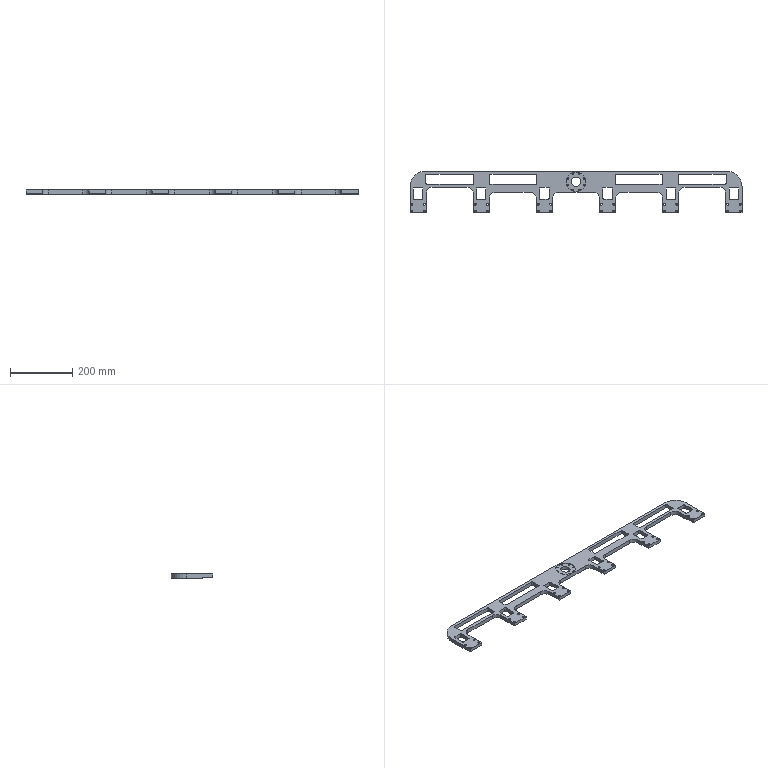NC program | NX | posted with a generic post | part box 1068 x 134 x 13 mm
Lines 1285 to 2457 of 4175:
(ZLEVEL_PROFILE_COPY_1_COPY_COPY , TOOL : D6)
N2526 T06 M6
N2528 G54
N2530 G17 G0 G90 X477.721 Y29.2 S9500 M3
N2532 G43 Z30. H6
N2534 Z-0.591
N2536 G94 G1 Y28.003 F1000.
N2538 X477.784 Y28.
N2540 X480. F1650.
N2542 Y30.216
N2544 X479.997 Y30.279
N2546 X478.8
N2548 G0 X477.721 Y29.2 Z-1.182
N2550 G1 Y28.003 F1000.
N2552 X477.784 Y28.
N2554 X480. F1650.
N2556 Y30.216
N2558 X479.997 Y30.279
N2560 X478.8
N2562 G0 X477.721 Y29.2 Z-1.773
N2564 G1 Y28.003 F1000.
N2566 X477.784 Y28.
N2568 X480. F1650.
N2570 Y30.216
N2572 X479.997 Y30.279
N2574 X478.8
N2576 G0 X477.721 Y29.2 Z-2.364
N2578 G1 Y28.003 F1000.
N2580 X477.784 Y28.
N2582 X480. F1650.
N2584 Y30.216
N2586 X479.997 Y30.279
N2588 X478.8
N2590 G0 X477.721 Y29.2 Z-2.955
N2592 G1 Y28.003 F1000.
N2594 X477.784 Y28.
N2596 X480. F1650.
N2598 Y30.216
N2600 X479.997 Y30.279
N2602 X478.8
N2604 G0 X477.721 Y29.2 Z-3.545
N2606 G1 Y28.003 F1000.
N2608 X477.784 Y28.
N2610 X480. F1650.
N2612 Y30.216
N2614 X479.997 Y30.279
N2616 X478.8
N2618 G0 X477.721 Y29.2 Z-4.136
N2620 G1 Y28.003 F1000.
N2622 X477.784 Y28.
N2624 X480. F1650.
N2626 Y30.216
N2628 X479.997 Y30.279
N2630 X478.8
N2632 G0 X477.721 Y29.2 Z-4.727
N2634 G1 Y28.003 F1000.
N2636 X477.784 Y28.
N2638 X480. F1650.
N2640 Y30.216
N2642 X479.997 Y30.279
N2644 X478.8
N2646 G0 X477.721 Y29.2 Z-5.318
N2648 G1 Y28.003 F1000.
N2650 X477.784 Y28.
N2652 X480. F1650.
N2654 Y30.216
N2656 X479.997 Y30.279
N2658 X478.8
N2660 G0 X477.721 Y29.2 Z-5.909
N2662 G1 Y28.003 F1000.
N2664 X477.784 Y28.
N2666 X480. F1650.
N2668 Y30.216
N2670 X479.997 Y30.279
N2672 X478.8
N2674 G0 X477.721 Y29.2 Z-6.5
N2676 G1 Y28.003 F1000.
N2678 X477.784 Y28.
N2680 X480. F1650.
N2682 Y30.216
N2684 X479.997 Y30.279
N2686 X478.8
N2688 G0 X477.721 Y29.2 Z-7.091
N2690 G1 Y28.003 F1000.
N2692 X477.784 Y28.
N2694 X480. F1650.
N2696 Y30.216
N2698 X479.997 Y30.279
N2700 X478.8
N2702 G0 X477.721 Y29.2 Z-7.682
N2704 G1 Y28.003 F1000.
N2706 X477.784 Y28.
N2708 X480. F1650.
N2710 Y30.216
N2712 X479.997 Y30.279
N2714 X478.8
N2716 G0 X477.709 Y29.2 Z-8.273
N2718 G1 Y28.003 F1000.
N2720 X477.772 Y28.
N2722 X480. F1650.
N2724 Y30.218
N2726 X479.997 Y30.281
N2728 X478.8
N2730 G0 X477.709 Y29.2 Z-8.864
N2732 G1 Y28.003 F1000.
N2734 X477.772 Y28.
N2736 X480. F1650.
N2738 Y30.218
N2740 X479.997 Y30.281
N2742 X478.8
N2744 G0 X477.709 Y29.2 Z-9.455
N2746 G1 Y28.003 F1000.
N2748 X477.772 Y28.
N2750 X480. F1650.
N2752 Y30.218
N2754 X479.997 Y30.281
N2756 X478.8
N2758 G0 X477.709 Y29.2 Z-10.045
N2760 G1 Y28.003 F1000.
N2762 X477.772 Y28.
N2764 X480. F1650.
N2766 Y30.218
N2768 X479.997 Y30.281
N2770 X478.8
N2772 G0 X477.709 Y29.2 Z-10.636
N2774 G1 Y28.003 F1000.
N2776 X477.772 Y28.
N2778 X480. F1650.
N2780 Y30.218
N2782 X479.997 Y30.281
N2784 X478.8
N2786 G0 X477.709 Y29.2 Z-11.227
N2788 G1 Y28.003 F1000.
N2790 X477.772 Y28.
N2792 X480. F1650.
N2794 Y30.218
N2796 X479.997 Y30.281
N2798 X478.8
N2800 G0 X477.709 Y29.2 Z-11.818
N2802 G1 Y28.003 F1000.
N2804 X477.772 Y28.
N2806 X480. F1650.
N2808 Y30.218
N2810 X479.997 Y30.281
N2812 X478.8
N2814 G0 X477.709 Y29.2 Z-12.409
N2816 G1 Y28.003 F1000.
N2818 X477.772 Y28.
N2820 X480. F1650.
N2822 Y30.218
N2824 X479.997 Y30.281
N2826 X478.8
N2828 G0 X477.709 Y29.2 Z-13.
N2830 G1 Y28.003 F1000.
N2832 X477.772 Y28.
N2834 X480. F1650.
N2836 Y30.218
N2838 X479.997 Y30.281
N2840 X478.8
N2842 G0 Z30.
N2844 Y51.721
N2846 Z-0.591
N2848 G1 X479.997 F1000.
N2850 X480. Y51.784
N2852 Y54. F1650.
N2854 X477.784
N2856 X477.721 Y53.997
N2858 Y52.8
N2860 G0 X478.8 Y51.721 Z-1.182
N2862 G1 X479.997 F1000.
N2864 X480. Y51.784
N2866 Y54. F1650.
N2868 X477.784
N2870 X477.721 Y53.997
N2872 Y52.8
N2874 G0 X478.8 Y51.721 Z-1.773
N2876 G1 X479.997 F1000.
N2878 X480. Y51.784
N2880 Y54. F1650.
N2882 X477.784
N2884 X477.721 Y53.997
N2886 Y52.8
N2888 G0 X478.8 Y51.721 Z-2.364
N2890 G1 X479.997 F1000.
N2892 X480. Y51.784
N2894 Y54. F1650.
N2896 X477.784
N2898 X477.721 Y53.997
N2900 Y52.8
N2902 G0 X478.8 Y51.721 Z-2.955
N2904 G1 X479.997 F1000.
N2906 X480. Y51.784
N2908 Y54. F1650.
N2910 X477.784
N2912 X477.721 Y53.997
N2914 Y52.8
N2916 G0 X478.8 Y51.721 Z-3.545
N2918 G1 X479.997 F1000.
N2920 X480. Y51.784
N2922 Y54. F1650.
N2924 X477.784
N2926 X477.721 Y53.997
N2928 Y52.8
N2930 G0 X478.8 Y51.721 Z-4.136
N2932 G1 X479.997 F1000.
N2934 X480. Y51.784
N2936 Y54. F1650.
N2938 X477.784
N2940 X477.721 Y53.997
N2942 Y52.8
N2944 G0 X478.8 Y51.721 Z-4.727
N2946 G1 X479.997 F1000.
N2948 X480. Y51.784
N2950 Y54. F1650.
N2952 X477.784
N2954 X477.721 Y53.997
N2956 Y52.8
N2958 G0 X478.8 Y51.721 Z-5.318
N2960 G1 X479.997 F1000.
N2962 X480. Y51.784
N2964 Y54. F1650.
N2966 X477.784
N2968 X477.721 Y53.997
N2970 Y52.8
N2972 G0 X478.8 Y51.721 Z-5.909
N2974 G1 X479.997 F1000.
N2976 X480. Y51.784
N2978 Y54. F1650.
N2980 X477.784
N2982 X477.721 Y53.997
N2984 Y52.8
N2986 G0 X478.8 Y51.721 Z-6.5
N2988 G1 X479.997 F1000.
N2990 X480. Y51.784
N2992 Y54. F1650.
N2994 X477.784
N2996 X477.721 Y53.997
N2998 Y52.8
N3000 G0 X478.8 Y51.721 Z-7.091
N3002 G1 X479.997 F1000.
N3004 X480. Y51.784
N3006 Y54. F1650.
N3008 X477.784
N3010 X477.721 Y53.997
N3012 Y52.8
N3014 G0 X478.8 Y51.721 Z-7.682
N3016 G1 X479.997 F1000.
N3018 X480. Y51.784
N3020 Y54. F1650.
N3022 X477.784
N3024 X477.721 Y53.997
N3026 Y52.8
N3028 G0 X478.8 Y51.73 Z-8.273
N3030 G1 X479.997 F1000.
N3032 X480. Y51.793
N3034 Y53.988 F1650.
N3036 Y54.
N3038 X477.795
N3040 X477.732 Y53.997
N3042 Y52.8
N3044 G0 X478.8 Y51.73 Z-8.864
N3046 G1 X479.997 F1000.
N3048 X480. Y51.793
N3050 Y53.988 F1650.
N3052 Y54.
N3054 X477.795
N3056 X477.732 Y53.997
N3058 Y52.8
N3060 G0 X478.8 Y51.73 Z-9.455
N3062 G1 X479.997 F1000.
N3064 X480. Y51.793
N3066 Y53.988 F1650.
N3068 Y54.
N3070 X477.795
N3072 X477.732 Y53.997
N3074 Y52.8
N3076 G0 X478.8 Y51.73 Z-10.045
N3078 G1 X479.997 F1000.
N3080 X480. Y51.793
N3082 Y53.988 F1650.
N3084 Y54.
N3086 X477.795
N3088 X477.732 Y53.997
N3090 Y52.8
N3092 G0 X478.8 Y51.73 Z-10.636
N3094 G1 X479.997 F1000.
N3096 X480. Y51.793
N3098 Y53.988 F1650.
N3100 Y54.
N3102 X477.795
N3104 X477.732 Y53.997
N3106 Y52.8
N3108 G0 X478.8 Y51.73 Z-11.227
N3110 G1 X479.997 F1000.
N3112 X480. Y51.793
N3114 Y53.988 F1650.
N3116 Y54.
N3118 X477.795
N3120 X477.732 Y53.997
N3122 Y52.8
N3124 G0 X478.8 Y51.73 Z-11.818
N3126 G1 X479.997 F1000.
N3128 X480. Y51.793
N3130 Y53.988 F1650.
N3132 Y54.
N3134 X477.795
N3136 X477.732 Y53.997
N3138 Y52.8
N3140 G0 X478.8 Y51.73 Z-12.409
N3142 G1 X479.997 F1000.
N3144 X480. Y51.793
N3146 Y53.988 F1650.
N3148 Y54.
N3150 X477.795
N3152 X477.732 Y53.997
N3154 Y52.8
N3156 G0 X478.8 Y51.73 Z-13.
N3158 G1 X479.997 F1000.
N3160 X480. Y51.793
N3162 Y53.988 F1650.
N3164 Y54.
N3166 X477.795
N3168 X477.732 Y53.997
N3170 Y52.8
N3172 G0 Z30.
N3174 X335.079
N3176 Z-0.591
N3178 G1 Y53.997 F1000.
N3180 X335.016 Y54.
N3182 X332.8 F1650.
N3184 Y51.784
N3186 X332.803 Y51.721
N3188 X334.
N3190 G0 X335.079 Y52.8 Z-1.182
N3192 G1 Y53.997 F1000.
N3194 X335.016 Y54.
N3196 X332.8 F1650.
N3198 Y51.784
N3200 X332.803 Y51.721
N3202 X334.
N3204 G0 X335.079 Y52.8 Z-1.773
N3206 G1 Y53.997 F1000.
N3208 X335.016 Y54.
N3210 X332.8 F1650.
N3212 Y51.784
N3214 X332.803 Y51.721
N3216 X334.
N3218 G0 X335.079 Y52.8 Z-2.364
N3220 G1 Y53.997 F1000.
N3222 X335.016 Y54.
N3224 X332.8 F1650.
N3226 Y51.784
N3228 X332.803 Y51.721
N3230 X334.
N3232 G0 X335.079 Y52.8 Z-2.955
N3234 G1 Y53.997 F1000.
N3236 X335.016 Y54.
N3238 X332.8 F1650.
N3240 Y51.784
N3242 X332.803 Y51.721
N3244 X334.
N3246 G0 X335.079 Y52.8 Z-3.545
N3248 G1 Y53.997 F1000.
N3250 X335.016 Y54.
N3252 X332.8 F1650.
N3254 Y51.784
N3256 X332.803 Y51.721
N3258 X334.
N3260 G0 X335.079 Y52.8 Z-4.136
N3262 G1 Y53.997 F1000.
N3264 X335.016 Y54.
N3266 X332.8 F1650.
N3268 Y51.784
N3270 X332.803 Y51.721
N3272 X334.
N3274 G0 X335.079 Y52.8 Z-4.727
N3276 G1 Y53.997 F1000.
N3278 X335.016 Y54.
N3280 X332.8 F1650.
N3282 Y51.784
N3284 X332.803 Y51.721
N3286 X334.
N3288 G0 X335.079 Y52.8 Z-5.318
N3290 G1 Y53.997 F1000.
N3292 X335.016 Y54.
N3294 X332.8 F1650.
N3296 Y51.784
N3298 X332.803 Y51.721
N3300 X334.
N3302 G0 X335.079 Y52.8 Z-5.909
N3304 G1 Y53.997 F1000.
N3306 X335.016 Y54.
N3308 X332.8 F1650.
N3310 Y51.784
N3312 X332.803 Y51.721
N3314 X334.
N3316 G0 X335.079 Y52.8 Z-6.5
N3318 G1 Y53.997 F1000.
N3320 X335.016 Y54.
N3322 X332.8 F1650.
N3324 Y51.784
N3326 X332.803 Y51.721
N3328 X334.
N3330 G0 X335.079 Y52.8 Z-7.091
N3332 G1 Y53.997 F1000.
N3334 X335.016 Y54.
N3336 X332.8 F1650.
N3338 Y51.784
N3340 X332.803 Y51.721
N3342 X334.
N3344 G0 X335.079 Y52.8 Z-7.682
N3346 G1 Y53.997 F1000.
N3348 X335.016 Y54.
N3350 X332.8 F1650.
N3352 Y51.784
N3354 X332.803 Y51.721
N3356 X334.
N3358 G0 X335.076 Y52.8 Z-8.273
N3360 G1 Y53.997 F1000.
N3362 X335.013 Y54.
N3364 X332.8 F1650.
N3366 Y51.774
N3368 X332.803 Y51.711
N3370 X334.
N3372 G0 X335.076 Y52.8 Z-8.864
N3374 G1 Y53.997 F1000.
N3376 X335.013 Y54.
N3378 X332.8 F1650.
N3380 Y51.774
N3382 X332.803 Y51.711
N3384 X334.
N3386 G0 X335.076 Y52.8 Z-9.455
N3388 G1 Y53.997 F1000.
N3390 X335.013 Y54.
N3392 X332.8 F1650.
N3394 Y51.774
N3396 X332.803 Y51.711
N3398 X334.
N3400 G0 X335.076 Y52.8 Z-10.045
N3402 G1 Y53.997 F1000.
N3404 X335.013 Y54.
N3406 X332.8 F1650.
N3408 Y51.774
N3410 X332.803 Y51.711
N3412 X334.
N3414 G0 X335.076 Y52.8 Z-10.636
N3416 G1 Y53.997 F1000.
N3418 X335.013 Y54.
N3420 X332.8 F1650.
N3422 Y51.774
N3424 X332.803 Y51.711
N3426 X334.
N3428 G0 X335.076 Y52.8 Z-11.227
N3430 G1 Y53.997 F1000.
N3432 X335.013 Y54.
N3434 X332.8 F1650.
N3436 Y51.774
N3438 X332.803 Y51.711
N3440 X334.
N3442 G0 X335.076 Y52.8 Z-11.818
N3444 G1 Y53.997 F1000.
N3446 X335.013 Y54.
N3448 X332.8 F1650.
N3450 Y51.774
N3452 X332.803 Y51.711
N3454 X334.
N3456 G0 X335.076 Y52.8 Z-12.409
N3458 G1 Y53.997 F1000.
N3460 X335.013 Y54.
N3462 X332.8 F1650.
N3464 Y51.774
N3466 X332.803 Y51.711
N3468 X334.
N3470 G0 X335.076 Y52.8 Z-13.
N3472 G1 Y53.997 F1000.
N3474 X335.013 Y54.
N3476 X332.8 F1650.
N3478 Y51.774
N3480 X332.803 Y51.711
N3482 X334.
N3484 G0 Z30.
N3486 Y30.279
N3488 Z-0.591
N3490 G1 X332.803 F1000.
N3492 X332.8 Y30.216
N3494 Y28. F1650.
N3496 X335.016
N3498 X335.079 Y28.003
N3500 Y29.2
N3502 G0 X334. Y30.279 Z-1.182
N3504 G1 X332.803 F1000.
N3506 X332.8 Y30.216
N3508 Y28. F1650.
N3510 X335.016
N3512 X335.079 Y28.003
N3514 Y29.2
N3516 G0 X334. Y30.279 Z-1.773
N3518 G1 X332.803 F1000.
N3520 X332.8 Y30.216
N3522 Y28. F1650.
N3524 X335.016
N3526 X335.079 Y28.003
N3528 Y29.2
N3530 G0 X334. Y30.279 Z-2.364
N3532 G1 X332.803 F1000.
N3534 X332.8 Y30.216
N3536 Y28. F1650.
N3538 X335.016
N3540 X335.079 Y28.003
N3542 Y29.2
N3544 G0 X334. Y30.279 Z-2.955
N3546 G1 X332.803 F1000.
N3548 X332.8 Y30.216
N3550 Y28. F1650.
N3552 X335.016
N3554 X335.079 Y28.003
N3556 Y29.2
N3558 G0 X334. Y30.279 Z-3.545
N3560 G1 X332.803 F1000.
N3562 X332.8 Y30.216
N3564 Y28. F1650.
N3566 X335.016
N3568 X335.079 Y28.003
N3570 Y29.2
N3572 G0 X334. Y30.279 Z-4.136
N3574 G1 X332.803 F1000.
N3576 X332.8 Y30.216
N3578 Y28. F1650.
N3580 X335.016
N3582 X335.079 Y28.003
N3584 Y29.2
N3586 G0 X334. Y30.279 Z-4.727
N3588 G1 X332.803 F1000.
N3590 X332.8 Y30.216
N3592 Y28. F1650.
N3594 X335.016
N3596 X335.079 Y28.003
N3598 Y29.2
N3600 G0 X334. Y30.279 Z-5.318
N3602 G1 X332.803 F1000.
N3604 X332.8 Y30.216
N3606 Y28. F1650.
N3608 X335.016
N3610 X335.079 Y28.003
N3612 Y29.2
N3614 G0 X334. Y30.279 Z-5.909
N3616 G1 X332.803 F1000.
N3618 X332.8 Y30.216
N3620 Y28. F1650.
N3622 X335.016
N3624 X335.079 Y28.003
N3626 Y29.2
N3628 G0 X334. Y30.279 Z-6.5
N3630 G1 X332.803 F1000.
N3632 X332.8 Y30.216
N3634 Y28. F1650.
N3636 X335.016
N3638 X335.079 Y28.003
N3640 Y29.2
N3642 G0 X334. Y30.279 Z-7.091
N3644 G1 X332.803 F1000.
N3646 X332.8 Y30.216
N3648 Y28. F1650.
N3650 X335.016
N3652 X335.079 Y28.003
N3654 Y29.2
N3656 G0 X334. Y30.279 Z-7.682
N3658 G1 X332.803 F1000.
N3660 X332.8 Y30.216
N3662 Y28. F1650.
N3664 X335.016
N3666 X335.079 Y28.003
N3668 Y29.2
N3670 G0 X334. Y30.279 Z-8.273
N3672 G1 X332.803 F1000.
N3674 X332.8 Y30.216
N3676 Y28. F1650.
N3678 X335.016
N3680 X335.079 Y28.003
N3682 Y29.2
N3684 G0 X334. Y30.279 Z-8.864
N3686 G1 X332.803 F1000.
N3688 X332.8 Y30.216
N3690 Y28. F1650.
N3692 X335.016
N3694 X335.079 Y28.003
N3696 Y29.2
N3698 G0 X334. Y30.279 Z-9.455
N3700 G1 X332.803 F1000.
N3702 X332.8 Y30.216
N3704 Y28. F1650.
N3706 X335.016
N3708 X335.079 Y28.003
N3710 Y29.2
N3712 G0 X334. Y30.279 Z-10.045
N3714 G1 X332.803 F1000.
N3716 X332.8 Y30.216
N3718 Y28. F1650.
N3720 X335.016
N3722 X335.079 Y28.003
N3724 Y29.2
N3726 G0 X334. Y30.279 Z-10.636
N3728 G1 X332.803 F1000.
N3730 X332.8 Y30.216
N3732 Y28. F1650.
N3734 X335.016
N3736 X335.079 Y28.003
N3738 Y29.2
N3740 G0 X334. Y30.279 Z-11.227
N3742 G1 X332.803 F1000.
N3744 X332.8 Y30.216
N3746 Y28. F1650.
N3748 X335.016
N3750 X335.079 Y28.003
N3752 Y29.2
N3754 G0 X334. Y30.279 Z-11.818
N3756 G1 X332.803 F1000.
N3758 X332.8 Y30.216
N3760 Y28. F1650.
N3762 X335.016
N3764 X335.079 Y28.003
N3766 Y29.2
N3768 G0 X334. Y30.279 Z-12.409
N3770 G1 X332.803 F1000.
N3772 X332.8 Y30.216
N3774 Y28. F1650.
N3776 X335.016
N3778 X335.079 Y28.003
N3780 Y29.2
N3782 G0 X334. Y30.279 Z-13.
N3784 G1 X332.803 F1000.
N3786 X332.8 Y30.216
N3788 Y28. F1650.
N3790 X335.016
N3792 X335.079 Y28.003
N3794 Y29.2
N3796 G0 Z30.
N3798 X274.521
N3800 Z-0.591
N3802 G1 Y28.003 F1000.
N3804 X274.584 Y28.
N3806 X276.8 F1650.
N3808 Y30.216
N3810 X276.797 Y30.279
N3812 X275.6
N3814 G0 X274.521 Y29.2 Z-1.182
N3816 G1 Y28.003 F1000.
N3818 X274.584 Y28.
N3820 X276.8 F1650.
N3822 Y30.216
N3824 X276.797 Y30.279
N3826 X275.6
N3828 G0 X274.521 Y29.2 Z-1.773
N3830 G1 Y28.003 F1000.
N3832 X274.584 Y28.
N3834 X276.8 F1650.
N3836 Y30.216
N3838 X276.797 Y30.279
N3840 X275.6
N3842 G0 X274.521 Y29.2 Z-2.364
N3844 G1 Y28.003 F1000.
N3846 X274.584 Y28.
N3848 X276.8 F1650.
N3850 Y30.216
N3852 X276.797 Y30.279
N3854 X275.6
N3856 G0 X274.521 Y29.2 Z-2.955
N3858 G1 Y28.003 F1000.
N3860 X274.584 Y28.
N3862 X276.8 F1650.
N3864 Y30.216
N3866 X276.797 Y30.279
N3868 X275.6
N3870 G0 X274.521 Y29.2 Z-3.545
N3872 G1 Y28.003 F1000.
N3874 X274.584 Y28.
N3876 X276.8 F1650.
N3878 Y30.216
N3880 X276.797 Y30.279
N3882 X275.6
N3884 G0 X274.521 Y29.2 Z-4.136
N3886 G1 Y28.003 F1000.
N3888 X274.584 Y28.
N3890 X276.8 F1650.
N3892 Y30.216
N3894 X276.797 Y30.279
N3896 X275.6
N3898 G0 X274.521 Y29.2 Z-4.727
N3900 G1 Y28.003 F1000.
N3902 X274.584 Y28.
N3904 X276.8 F1650.
N3906 Y30.216
N3908 X276.797 Y30.279
N3910 X275.6
N3912 G0 X274.521 Y29.2 Z-5.318
N3914 G1 Y28.003 F1000.
N3916 X274.584 Y28.
N3918 X276.8 F1650.
N3920 Y30.216
N3922 X276.797 Y30.279
N3924 X275.6
N3926 G0 X274.521 Y29.2 Z-5.909
N3928 G1 Y28.003 F1000.
N3930 X274.584 Y28.
N3932 X276.8 F1650.
N3934 Y30.216
N3936 X276.797 Y30.279
N3938 X275.6
N3940 G0 X274.521 Y29.2 Z-6.5
N3942 G1 Y28.003 F1000.
N3944 X274.584 Y28.
N3946 X276.8 F1650.
N3948 Y30.216
N3950 X276.797 Y30.279
N3952 X275.6
N3954 G0 X274.521 Y29.2 Z-7.091
N3956 G1 Y28.003 F1000.
N3958 X274.584 Y28.
N3960 X276.8 F1650.
N3962 Y30.216
N3964 X276.797 Y30.279
N3966 X275.6
N3968 G0 X274.521 Y29.2 Z-7.682
N3970 G1 Y28.003 F1000.
N3972 X274.584 Y28.
N3974 X276.8 F1650.
N3976 Y30.216
N3978 X276.797 Y30.279
N3980 X275.6
N3982 G0 X274.507 Y29.2 Z-8.273
N3984 G1 Y28.003 F1000.
N3986 X274.569 Y28.
N3988 X276.8 F1650.
N3990 Y30.217
N3992 X276.797 Y30.28
N3994 X275.6
N3996 G0 X274.507 Y29.2 Z-8.864
N3998 G1 Y28.003 F1000.
N4000 X274.569 Y28.
N4002 X276.8 F1650.
N4004 Y30.217
N4006 X276.797 Y30.28
N4008 X275.6
N4010 G0 X274.507 Y29.2 Z-9.455
N4012 G1 Y28.003 F1000.
N4014 X274.569 Y28.
N4016 X276.8 F1650.
N4018 Y30.217
N4020 X276.797 Y30.28
N4022 X275.6
N4024 G0 X274.507 Y29.2 Z-10.045
N4026 G1 Y28.003 F1000.
N4028 X274.569 Y28.
N4030 X276.8 F1650.
N4032 Y30.217
N4034 X276.797 Y30.28
N4036 X275.6
N4038 G0 X274.507 Y29.2 Z-10.636
N4040 G1 Y28.003 F1000.
N4042 X274.569 Y28.
N4044 X276.8 F1650.
N4046 Y30.217
N4048 X276.797 Y30.28
N4050 X275.6
N4052 G0 X274.507 Y29.2 Z-11.227
N4054 G1 Y28.003 F1000.
N4056 X274.569 Y28.
N4058 X276.8 F1650.
N4060 Y30.217
N4062 X276.797 Y30.28
N4064 X275.6
N4066 G0 X274.507 Y29.2 Z-11.818
N4068 G1 Y28.003 F1000.
N4070 X274.569 Y28.
N4072 X276.8 F1650.
N4074 Y30.217
N4076 X276.797 Y30.28
N4078 X275.6
N4080 G0 X274.507 Y29.2 Z-12.409
N4082 G1 Y28.003 F1000.
N4084 X274.569 Y28.
N4086 X276.8 F1650.
N4088 Y30.217
N4090 X276.797 Y30.28
N4092 X275.6
N4094 G0 X274.507 Y29.2 Z-13.
N4096 G1 Y28.003 F1000.
N4098 X274.569 Y28.
N4100 X276.8 F1650.
N4102 Y30.217
N4104 X276.797 Y30.28
N4106 X275.6
N4108 G0 Z30.
N4110 Y51.721
N4112 Z-0.591
N4114 G1 X276.797 F1000.
N4116 X276.8 Y51.784
N4118 Y54. F1650.
N4120 X274.584
N4122 X274.521 Y53.997
N4124 Y52.8
N4126 G0 X275.6 Y51.721 Z-1.182
N4128 G1 X276.797 F1000.
N4130 X276.8 Y51.784
N4132 Y54. F1650.
N4134 X274.584
N4136 X274.521 Y53.997
N4138 Y52.8
N4140 G0 X275.6 Y51.721 Z-1.773
N4142 G1 X276.797 F1000.
N4144 X276.8 Y51.784
N4146 Y54. F1650.
N4148 X274.584
N4150 X274.521 Y53.997
N4152 Y52.8
N4154 G0 X275.6 Y51.721 Z-2.364
N4156 G1 X276.797 F1000.
N4158 X276.8 Y51.784
N4160 Y54. F1650.
N4162 X274.584
N4164 X274.521 Y53.997
N4166 Y52.8
N4168 G0 X275.6 Y51.721 Z-2.955
N4170 G1 X276.797 F1000.
N4172 X276.8 Y51.784
N4174 Y54. F1650.
N4176 X274.584
N4178 X274.521 Y53.997
N4180 Y52.8
N4182 G0 X275.6 Y51.721 Z-3.545
N4184 G1 X276.797 F1000.
N4186 X276.8 Y51.784
N4188 Y54. F1650.
N4190 X274.584
N4192 X274.521 Y53.997
N4194 Y52.8
N4196 G0 X275.6 Y51.721 Z-4.136
N4198 G1 X276.797 F1000.
N4200 X276.8 Y51.784
N4202 Y54. F1650.
N4204 X274.584
N4206 X274.521 Y53.997
N4208 Y52.8
N4210 G0 X275.6 Y51.721 Z-4.727
N4212 G1 X276.797 F1000.
N4214 X276.8 Y51.784
N4216 Y54. F1650.
N4218 X274.584
N4220 X274.521 Y53.997
N4222 Y52.8
N4224 G0 X275.6 Y51.721 Z-5.318
N4226 G1 X276.797 F1000.
N4228 X276.8 Y51.784
N4230 Y54. F1650.
N4232 X274.584
N4234 X274.521 Y53.997
N4236 Y52.8
N4238 G0 X275.6 Y51.721 Z-5.909
N4240 G1 X276.797 F1000.
N4242 X276.8 Y51.784
N4244 Y54. F1650.
N4246 X274.584
N4248 X274.521 Y53.997
N4250 Y52.8
N4252 G0 X275.6 Y51.721 Z-6.5
N4254 G1 X276.797 F1000.
N4256 X276.8 Y51.784
N4258 Y54. F1650.
N4260 X274.584
N4262 X274.521 Y53.997
N4264 Y52.8
N4266 G0 X275.6 Y51.721 Z-7.091
N4268 G1 X276.797 F1000.
N4270 X276.8 Y51.784
N4272 Y54. F1650.
N4274 X274.584
N4276 X274.521 Y53.997
N4278 Y52.8
N4280 G0 X275.6 Y51.721 Z-7.682
N4282 G1 X276.797 F1000.
N4284 X276.8 Y51.784
N4286 Y54. F1650.
N4288 X274.584
N4290 X274.521 Y53.997
N4292 Y52.8
N4294 G0 X275.6 Y51.731 Z-8.273
N4296 G1 X276.797 F1000.
N4298 X276.8 Y51.794
N4300 Y53.988 F1650.
N4302 Y54.
N4304 X274.593
N4306 X274.531 Y53.997
N4308 Y52.8
N4310 G0 X275.6 Y51.731 Z-8.864
N4312 G1 X276.797 F1000.
N4314 X276.8 Y51.794
N4316 Y53.988 F1650.
N4318 Y54.
N4320 X274.593
N4322 X274.531 Y53.997
N4324 Y52.8
N4326 G0 X275.6 Y51.731 Z-9.455
N4328 G1 X276.797 F1000.
N4330 X276.8 Y51.794
N4332 Y53.988 F1650.
N4334 Y54.
N4336 X274.593
N4338 X274.531 Y53.997
N4340 Y52.8
N4342 G0 X275.6 Y51.731 Z-10.045
N4344 G1 X276.797 F1000.
N4346 X276.8 Y51.794
N4348 Y53.988 F1650.
N4350 Y54.
N4352 X274.593
N4354 X274.531 Y53.997
N4356 Y52.8
N4358 G0 X275.6 Y51.731 Z-10.636
N4360 G1 X276.797 F1000.
N4362 X276.8 Y51.794
N4364 Y53.988 F1650.
N4366 Y54.
N4368 X274.593
N4370 X274.531 Y53.997
N4372 Y52.8
N4374 G0 X275.6 Y51.731 Z-11.227
N4376 G1 X276.797 F1000.
N4378 X276.8 Y51.794
N4380 Y53.988 F1650.
N4382 Y54.
N4384 X274.593
N4386 X274.531 Y53.997
N4388 Y52.8
N4390 G0 X275.6 Y51.731 Z-11.818
N4392 G1 X276.797 F1000.
N4394 X276.8 Y51.794
N4396 Y53.988 F1650.
N4398 Y54.
N4400 X274.593
N4402 X274.531 Y53.997
N4404 Y52.8
N4406 G0 X275.6 Y51.731 Z-12.409
N4408 G1 X276.797 F1000.
N4410 X276.8 Y51.794
N4412 Y53.988 F1650.
N4414 Y54.
N4416 X274.593
N4418 X274.531 Y53.997
N4420 Y52.8
N4422 G0 X275.6 Y51.731 Z-13.
N4424 G1 X276.797 F1000.
N4426 X276.8 Y51.794
N4428 Y53.988 F1650.
N4430 Y54.
N4432 X274.593
N4434 X274.531 Y53.997
N4436 Y52.8
N4438 G0 Z30.
N4440 X131.879
N4442 Z-0.591
N4444 G1 Y53.997 F1000.
N4446 X131.816 Y54.
N4448 X129.6 F1650.
N4450 Y51.784
N4452 X129.603 Y51.721
N4454 X130.8
N4456 G0 X131.879 Y52.8 Z-1.182
N4458 G1 Y53.997 F1000.
N4460 X131.816 Y54.
N4462 X129.6 F1650.
N4464 Y51.784
N4466 X129.603 Y51.721
N4468 X130.8
N4470 G0 X131.879 Y52.8 Z-1.773
N4472 G1 Y53.997 F1000.
N4474 X131.816 Y54.
N4476 X129.6 F1650.
N4478 Y51.784
N4480 X129.603 Y51.721
N4482 X130.8
N4484 G0 X131.879 Y52.8 Z-2.364
N4486 G1 Y53.997 F1000.
N4488 X131.816 Y54.
N4490 X129.6 F1650.
N4492 Y51.784
N4494 X129.603 Y51.721
N4496 X130.8
N4498 G0 X131.879 Y52.8 Z-2.955
N4500 G1 Y53.997 F1000.
N4502 X131.816 Y54.
N4504 X129.6 F1650.
N4506 Y51.784
N4508 X129.603 Y51.721
N4510 X130.8
N4512 G0 X131.879 Y52.8 Z-3.545
N4514 G1 Y53.997 F1000.
N4516 X131.816 Y54.
N4518 X129.6 F1650.
N4520 Y51.784
N4522 X129.603 Y51.721
N4524 X130.8
N4526 G0 X131.879 Y52.8 Z-4.136
N4528 G1 Y53.997 F1000.
N4530 X131.816 Y54.
N4532 X129.6 F1650.
N4534 Y51.784
N4536 X129.603 Y51.721
N4538 X130.8
N4540 G0 X131.879 Y52.8 Z-4.727
N4542 G1 Y53.997 F1000.
N4544 X131.816 Y54.
N4546 X129.6 F1650.
N4548 Y51.784
N4550 X129.603 Y51.721
N4552 X130.8
N4554 G0 X131.879 Y52.8 Z-5.318
N4556 G1 Y53.997 F1000.
N4558 X131.816 Y54.
N4560 X129.6 F1650.
N4562 Y51.784
N4564 X129.603 Y51.721
N4566 X130.8
N4568 G0 X131.879 Y52.8 Z-5.909
N4570 G1 Y53.997 F1000.
N4572 X131.816 Y54.
N4574 X129.6 F1650.
N4576 Y51.784
N4578 X129.603 Y51.721
N4580 X130.8
N4582 G0 X131.879 Y52.8 Z-6.5
N4584 G1 Y53.997 F1000.
N4586 X131.816 Y54.
N4588 X129.6 F1650.
N4590 Y51.784
N4592 X129.603 Y51.721
N4594 X130.8
N4596 G0 X131.879 Y52.8 Z-7.091
N4598 G1 Y53.997 F1000.
N4600 X131.816 Y54.
N4602 X129.6 F1650.
N4604 Y51.784
N4606 X129.603 Y51.721
N4608 X130.8
N4610 G0 X131.879 Y52.8 Z-7.682
N4612 G1 Y53.997 F1000.
N4614 X131.816 Y54.
N4616 X129.6 F1650.
N4618 Y51.784
N4620 X129.603 Y51.721
N4622 X130.8
N4624 G0 X131.872 Y52.8 Z-8.273
N4626 G1 Y53.997 F1000.
N4628 X131.81 Y54.
N4630 X129.6 F1650.
N4632 Y51.782
N4634 X129.603 Y51.72
N4636 X130.8
N4638 G0 X131.872 Y52.8 Z-8.864
N4640 G1 Y53.997 F1000.
N4642 X131.81 Y54.
N4644 X129.6 F1650.
N4646 Y51.782
N4648 X129.603 Y51.72
N4650 X130.8
N4652 G0 X131.872 Y52.8 Z-9.455
N4654 G1 Y53.997 F1000.
N4656 X131.81 Y54.
N4658 X129.6 F1650.
N4660 Y51.782
N4662 X129.603 Y51.72
N4664 X130.8
N4666 G0 X131.872 Y52.8 Z-10.045
N4668 G1 Y53.997 F1000.
N4670 X131.81 Y54.
N4672 X129.6 F1650.
N4674 Y51.782
N4676 X129.603 Y51.72
N4678 X130.8
N4680 G0 X131.872 Y52.8 Z-10.636
N4682 G1 Y53.997 F1000.
N4684 X131.81 Y54.
N4686 X129.6 F1650.
N4688 Y51.782
N4690 X129.603 Y51.72
N4692 X130.8
N4694 G0 X131.872 Y52.8 Z-11.227
N4696 G1 Y53.997 F1000.
N4698 X131.81 Y54.
N4700 X129.6 F1650.
N4702 Y51.782
N4704 X129.603 Y51.72
N4706 X130.8
N4708 G0 X131.872 Y52.8 Z-11.818
N4710 G1 Y53.997 F1000.
N4712 X131.81 Y54.
N4714 X129.6 F1650.
N4716 Y51.782
N4718 X129.603 Y51.72
N4720 X130.8
N4722 G0 X131.872 Y52.8 Z-12.409
N4724 G1 Y53.997 F1000.
N4726 X131.81 Y54.
N4728 X129.6 F1650.
N4730 Y51.782
N4732 X129.603 Y51.72
N4734 X130.8
N4736 G0 X131.872 Y52.8 Z-13.
N4738 G1 Y53.997 F1000.
N4740 X131.81 Y54.
N4742 X129.6 F1650.
N4744 Y51.782
N4746 X129.603 Y51.72
N4748 X130.8
N4750 G0 Z30.
N4752 Y30.279
N4754 Z-0.591
N4756 G1 X129.603 F1000.
N4758 X129.6 Y30.216
N4760 Y28. F1650.
N4762 X131.816
N4764 X131.879 Y28.003
N4766 Y29.2
N4768 G0 X130.8 Y30.279 Z-1.182
N4770 G1 X129.603 F1000.
N4772 X129.6 Y30.216
N4774 Y28. F1650.
N4776 X131.816
N4778 X131.879 Y28.003
N4780 Y29.2
N4782 G0 X130.8 Y30.279 Z-1.773
N4784 G1 X129.603 F1000.
N4786 X129.6 Y30.216
N4788 Y28. F1650.
N4790 X131.816
N4792 X131.879 Y28.003
N4794 Y29.2
N4796 G0 X130.8 Y30.279 Z-2.364
N4798 G1 X129.603 F1000.
N4800 X129.6 Y30.216
N4802 Y28. F1650.
N4804 X131.816
N4806 X131.879 Y28.003
N4808 Y29.2
N4810 G0 X130.8 Y30.279 Z-2.955
N4812 G1 X129.603 F1000.
N4814 X129.6 Y30.216
N4816 Y28. F1650.
N4818 X131.816
N4820 X131.879 Y28.003
N4822 Y29.2
N4824 G0 X130.8 Y30.279 Z-3.545
N4826 G1 X129.603 F1000.
N4828 X129.6 Y30.216
N4830 Y28. F1650.
N4832 X131.816
N4834 X131.879 Y28.003
N4836 Y29.2
N4838 G0 X130.8 Y30.279 Z-4.136
N4840 G1 X129.603 F1000.
N4842 X129.6 Y30.216
N4844 Y28. F1650.
N4846 X131.816
N4848 X131.879 Y28.003
N4850 Y29.2
N4852 G0 X130.8 Y30.279 Z-4.727
N4854 G1 X129.603 F1000.
N4856 X129.6 Y30.216
N4858 Y28. F1650.
N4860 X131.816
N4862 X131.879 Y28.003
N4864 Y29.2